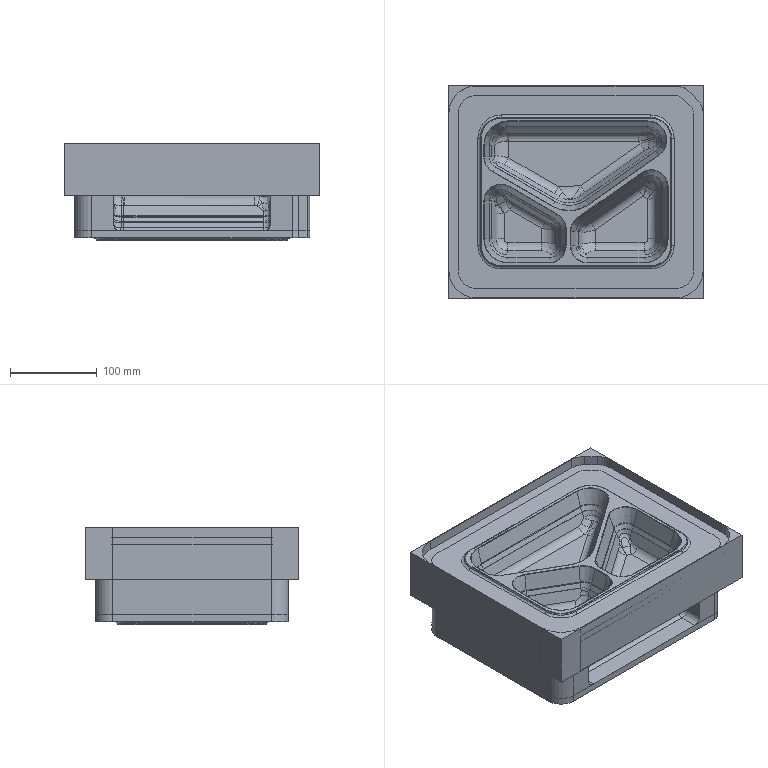NC program | NX | posted with a generic post | part box 295.651 x 246.652 x 112.895 mm
Lines 269047 to 269786 of 299251:
(D5 , TOOL : D10)
N538074 M6
N538076 G53
N538078 G17 G0 G90 X140.272 Y-100.089 S7000 M3 M8
N538080 G43 Z210.5 H0
N538082 Z50.884
N538084 G94 G1 X139.255 Y-102.613 Z50.741 F4000.
N538086 X137.526 Y-105.653 Z50.558
N538088 X135.406 Y-108.434 Z50.375
N538090 X132.933 Y-110.906 Z50.192
N538092 X130.152 Y-113.026 Z50.008
N538094 X127.113 Y-114.755 Z49.825
N538096 X123.869 Y-116.063 Z49.642
N538098 X120.48 Y-116.925 Z49.459
N538100 X117.007 Y-117.326 Z49.275
N538102 X109.541 Z48.884
N538104 X-115.756
N538106 G2 X-141.826 Y-91.256 R26.07
N538108 G1 Y91.256
N538110 G2 X-115.756 Y117.326 R26.07
N538112 G1 X115.613
N538114 G2 X126.951 Y112.629 R16.035
N538116 G1 X137.129 Y102.452
N538118 G2 X141.826 Y91.113 R16.035
N538120 G1 Y-91.256
N538122 G2 X115.756 Y-117.326 R26.07
N538124 G1 X109.541
N538126 Y-110.326
N538128 X-115.756
N538130 G2 X-134.826 Y-91.256 R19.07
N538132 G1 Y91.256
N538134 G2 X-115.756 Y110.326 R19.07
N538136 G1 X115.613
N538138 G2 X122.002 Y107.68 R9.035
N538140 G1 X132.179 Y97.502
N538142 G2 X134.826 Y91.113 R9.035
N538144 G1 Y-91.256
N538146 G2 X115.756 Y-110.326 R19.07
N538148 G1 X109.541
N538150 Y-103.326
N538152 X-115.756
N538154 G2 X-127.826 Y-91.256 R12.07
N538156 G1 Y91.256
N538158 G2 X-115.756 Y103.326 R12.07
N538160 G1 X115.613
N538162 G2 X117.052 Y102.73 R2.035
N538164 G1 X127.23 Y92.552
N538166 G2 X127.826 Y91.113 R2.035
N538168 G1 Y-91.256
N538170 G2 X115.756 Y-103.326 R12.07
N538172 G1 X109.541
N538174 Y-96.326
N538176 X-115.756
N538178 G2 X-120.826 Y-91.256 R5.07
N538180 G1 Y-80.756
N538182 X-113.826
N538184 G3 X-105.256 Y-89.326 R33.145
N538186 G1 X-113.826
N538188 Y-80.756
N538190 X-120.826
N538192 Y91.256
N538194 G2 X-115.756 Y96.326 R5.07
N538196 G1 X-105.256
N538198 Y89.326
N538200 G3 X-113.826 Y80.756 R33.145
N538202 G1 Y89.326
N538204 X-105.256
N538206 Y96.326
N538208 X113.556
N538210 X120.826 Y89.057
N538212 Y80.756
N538214 X113.826
N538216 G3 X105.256 Y89.326 R33.145
N538218 G1 X110.657
N538220 X113.826 Y86.157
N538222 Y80.756
N538224 X120.826
N538226 Y-91.256
N538228 G2 X115.756 Y-96.326 R5.07
N538230 G1 X109.541
N538232 Y-89.326
N538234 X105.256
N538236 G3 X113.826 Y-80.756 R33.145
N538238 G1 X112.671 Y-79.964
N538240 G2 X86.499 Y-93.744 R31.745
N538242 G1 X-86.499
N538244 G2 X-118.244 Y-61.999 R31.745
N538246 G1 Y61.999
N538248 G2 X-86.499 Y93.744 R31.745
N538250 G1 X86.499
N538252 G2 X118.244 Y61.999 R31.745
N538254 G1 Y-61.999
N538256 G2 X112.671 Y-79.964 R31.745
N538258 G1 X113.826 Y-80.756
N538260 Y-89.326
N538262 X109.541
N538264 G3 X107.541 Y-91.326 R2.
N538266 G1 Z49.884
N538268 G0 Z210.5
(D6 , TOOL : D10)
N538270 X-140.826 Y-74.472
N538272 Z49.884
N538274 G1 Y92.483 Z49.738
N538276 X-140.437 Y95.819 Z49.735
N538278 X-139.607 Y99.073 Z49.733
N538280 X-138.35 Y102.188 Z49.73
N538282 X-136.688 Y105.106 Z49.727
N538284 X-134.652 Y107.777 Z49.724
N538286 X-132.277 Y110.152 Z49.721
N538288 X-129.606 Y112.189 Z49.718
N538290 X-126.687 Y113.85 Z49.715
N538292 X-123.573 Y115.108 Z49.712
N538294 X-120.319 Y115.938 Z49.709
N538296 X-116.982 Y116.326 Z49.706
N538298 X116.563 Z49.502
N538300 X119.017 Y115.966 Z49.5
N538302 X121.378 Y115.209 Z49.498
N538304 X123.583 Y114.075 Z49.496
N538306 X125.572 Y112.594 Z49.494
N538308 X137.094 Y101.073 Z49.479
N538310 X138.575 Y99.084 Z49.477
N538312 X139.709 Y96.878 Z49.475
N538314 X140.466 Y94.517 Z49.473
N538316 X140.826 Y92.064 Z49.471
N538318 Y-92.483 Z49.31
N538320 X140.437 Y-95.819 Z49.307
N538322 X139.607 Y-99.073 Z49.304
N538324 X138.35 Y-102.188 Z49.301
N538326 X136.688 Y-105.106 Z49.298
N538328 X134.652 Y-107.777 Z49.295
N538330 X132.277 Y-110.152 Z49.292
N538332 X129.606 Y-112.189 Z49.289
N538334 X126.687 Y-113.85 Z49.286
N538336 X123.573 Y-115.108 Z49.283
N538338 X120.319 Y-115.938 Z49.28
N538340 X116.982 Y-116.326 Z49.278
N538342 X-116.982 Z49.073
N538344 X-120.319 Y-115.938 Z49.07
N538346 X-123.573 Y-115.108 Z49.067
N538348 X-126.687 Y-113.85 Z49.065
N538350 X-129.606 Y-112.189 Z49.062
N538352 X-132.277 Y-110.152 Z49.059
N538354 X-134.652 Y-107.777 Z49.056
N538356 X-136.688 Y-105.106 Z49.053
N538358 X-138.35 Y-102.188 Z49.05
N538360 X-139.607 Y-99.073 Z49.047
N538362 X-140.437 Y-95.819 Z49.044
N538364 X-140.826 Y-92.483 Z49.041
N538366 Y92.483 Z48.88
N538368 X-140.437 Y95.819 Z48.877
N538370 X-139.607 Y99.073 Z48.874
N538372 X-138.35 Y102.188 Z48.871
N538374 X-136.688 Y105.106 Z48.868
N538376 X-134.652 Y107.777 Z48.865
N538378 X-132.277 Y110.152 Z48.862
N538380 X-129.606 Y112.189 Z48.859
N538382 X-126.687 Y113.85 Z48.856
N538384 X-123.573 Y115.108 Z48.853
N538386 X-120.319 Y115.938 Z48.85
N538388 X-116.982 Y116.326 Z48.847
N538390 X116.563 Z48.644
N538392 X119.017 Y115.966 Z48.641
N538394 X121.378 Y115.209 Z48.639
N538396 X123.583 Y114.075 Z48.637
N538398 X125.572 Y112.594 Z48.635
N538400 X137.094 Y101.073 Z48.621
N538402 X138.575 Y99.084 Z48.619
N538404 X139.709 Y96.878 Z48.616
N538406 X140.466 Y94.517 Z48.614
N538408 X140.826 Y92.064 Z48.612
N538410 Y-92.483 Z48.451
N538412 X140.437 Y-95.819 Z48.448
N538414 X139.607 Y-99.073 Z48.445
N538416 X138.35 Y-102.188 Z48.442
N538418 X136.688 Y-105.106 Z48.439
N538420 X134.652 Y-107.777 Z48.436
N538422 X132.277 Y-110.152 Z48.433
N538424 X129.606 Y-112.189 Z48.431
N538426 X126.687 Y-113.85 Z48.428
N538428 X123.573 Y-115.108 Z48.425
N538430 X120.319 Y-115.938 Z48.422
N538432 X116.982 Y-116.326 Z48.419
N538434 X-116.982 Z48.215
N538436 X-120.319 Y-115.938 Z48.212
N538438 X-123.573 Y-115.108 Z48.209
N538440 X-126.687 Y-113.85 Z48.206
N538442 X-129.606 Y-112.189 Z48.203
N538444 X-132.277 Y-110.152 Z48.2
N538446 X-134.652 Y-107.777 Z48.197
N538448 X-136.688 Y-105.106 Z48.194
N538450 X-138.35 Y-102.188 Z48.191
N538452 X-139.607 Y-99.073 Z48.188
N538454 X-140.437 Y-95.819 Z48.185
N538456 X-140.826 Y-92.483 Z48.182
N538458 Y92.483 Z48.021
N538460 X-140.437 Y95.819 Z48.018
N538462 X-139.607 Y99.073 Z48.015
N538464 X-138.35 Y102.188 Z48.012
N538466 X-136.688 Y105.106 Z48.009
N538468 X-134.652 Y107.777 Z48.006
N538470 X-132.277 Y110.152 Z48.003
N538472 X-129.606 Y112.189 Z48.
N538474 X-126.687 Y113.85 Z47.998
N538476 X-123.573 Y115.108 Z47.995
N538478 X-120.319 Y115.938 Z47.992
N538480 X-116.982 Y116.326 Z47.989
N538482 X116.563 Z47.785
N538484 X119.017 Y115.966 Z47.783
N538486 X121.378 Y115.209 Z47.781
N538488 X123.583 Y114.075 Z47.778
N538490 X125.572 Y112.594 Z47.776
N538492 X137.094 Y101.073 Z47.762
N538494 X138.575 Y99.084 Z47.76
N538496 X139.709 Y96.878 Z47.758
N538498 X140.466 Y94.517 Z47.756
N538500 X140.826 Y92.064 Z47.753
N538502 Y-92.483 Z47.592
N538504 X140.437 Y-95.819 Z47.589
N538506 X139.607 Y-99.073 Z47.587
N538508 X138.35 Y-102.188 Z47.584
N538510 X136.688 Y-105.106 Z47.581
N538512 X134.652 Y-107.777 Z47.578
N538514 X132.277 Y-110.152 Z47.575
N538516 X129.606 Y-112.189 Z47.572
N538518 X126.687 Y-113.85 Z47.569
N538520 X123.573 Y-115.108 Z47.566
N538522 X120.319 Y-115.938 Z47.563
N538524 X116.982 Y-116.326 Z47.56
N538526 X-116.982 Z47.356
N538528 X-120.319 Y-115.938 Z47.353
N538530 X-123.573 Y-115.108 Z47.35
N538532 X-126.687 Y-113.85 Z47.347
N538534 X-129.606 Y-112.189 Z47.344
N538536 X-132.277 Y-110.152 Z47.341
N538538 X-134.652 Y-107.777 Z47.338
N538540 X-136.688 Y-105.106 Z47.335
N538542 X-138.35 Y-102.188 Z47.333
N538544 X-139.607 Y-99.073 Z47.33
N538546 X-140.437 Y-95.819 Z47.327
N538548 X-140.826 Y-92.483 Z47.324
N538550 Y92.483 Z47.162
N538552 X-140.437 Y95.819 Z47.159
N538554 X-139.607 Y99.073 Z47.156
N538556 X-138.35 Y102.188 Z47.154
N538558 X-136.688 Y105.106 Z47.151
N538560 X-134.652 Y107.777 Z47.148
N538562 X-132.277 Y110.152 Z47.145
N538564 X-129.606 Y112.189 Z47.142
N538566 X-126.687 Y113.85 Z47.139
N538568 X-123.573 Y115.108 Z47.136
N538570 X-120.319 Y115.938 Z47.133
N538572 X-116.982 Y116.326 Z47.13
N538574 X116.563 Z46.926
N538576 X119.017 Y115.966 Z46.924
N538578 X121.378 Y115.209 Z46.922
N538580 X123.583 Y114.075 Z46.92
N538582 X125.572 Y112.594 Z46.918
N538584 X137.094 Y101.073 Z46.903
N538586 X138.575 Y99.084 Z46.901
N538588 X139.709 Y96.878 Z46.899
N538590 X140.466 Y94.517 Z46.897
N538592 X140.826 Y92.064 Z46.895
N538594 Y-92.483 Z46.734
N538596 X140.437 Y-95.819 Z46.731
N538598 X139.607 Y-99.073 Z46.728
N538600 X138.35 Y-102.188 Z46.725
N538602 X136.688 Y-105.106 Z46.722
N538604 X134.652 Y-107.777 Z46.719
N538606 X132.277 Y-110.152 Z46.716
N538608 X129.606 Y-112.189 Z46.713
N538610 X126.687 Y-113.85 Z46.71
N538612 X123.573 Y-115.108 Z46.707
N538614 X120.319 Y-115.938 Z46.704
N538616 X116.982 Y-116.326 Z46.701
N538618 X-116.982 Z46.497
N538620 X-120.319 Y-115.938 Z46.494
N538622 X-123.573 Y-115.108 Z46.491
N538624 X-126.687 Y-113.85 Z46.488
N538626 X-129.606 Y-112.189 Z46.486
N538628 X-132.277 Y-110.152 Z46.483
N538630 X-134.652 Y-107.777 Z46.48
N538632 X-136.688 Y-105.106 Z46.477
N538634 X-138.35 Y-102.188 Z46.474
N538636 X-139.607 Y-99.073 Z46.471
N538638 X-140.437 Y-95.819 Z46.468
N538640 X-140.826 Y-92.483 Z46.465
N538642 Y92.483 Z46.304
N538644 X-140.437 Y95.819 Z46.301
N538646 X-139.607 Y99.073 Z46.298
N538648 X-138.35 Y102.188 Z46.295
N538650 X-136.688 Y105.106 Z46.292
N538652 X-134.652 Y107.777 Z46.289
N538654 X-132.277 Y110.152 Z46.286
N538656 X-129.606 Y112.189 Z46.283
N538658 X-126.687 Y113.85 Z46.28
N538660 X-123.573 Y115.108 Z46.277
N538662 X-120.319 Y115.938 Z46.274
N538664 X-116.982 Y116.326 Z46.271
N538666 X116.563 Z46.068
N538668 X119.017 Y115.966 Z46.065
N538670 X121.378 Y115.209 Z46.063
N538672 X123.583 Y114.075 Z46.061
N538674 X125.572 Y112.594 Z46.059
N538676 X137.094 Y101.073 Z46.045
N538678 X138.575 Y99.084 Z46.043
N538680 X139.709 Y96.878 Z46.04
N538682 X140.466 Y94.517 Z46.038
N538684 X140.826 Y92.064 Z46.036
N538686 Y-92.483 Z45.875
N538688 X140.437 Y-95.819 Z45.872
N538690 X139.607 Y-99.073 Z45.869
N538692 X138.35 Y-102.188 Z45.866
N538694 X136.688 Y-105.106 Z45.863
N538696 X134.652 Y-107.777 Z45.86
N538698 X132.277 Y-110.152 Z45.857
N538700 X129.606 Y-112.189 Z45.854
N538702 X126.687 Y-113.85 Z45.852
N538704 X123.573 Y-115.108 Z45.849
N538706 X120.319 Y-115.938 Z45.846
N538708 X116.982 Y-116.326 Z45.843
N538710 X-116.982 Z45.639
N538712 X-120.319 Y-115.938 Z45.636
N538714 X-123.573 Y-115.108 Z45.633
N538716 X-126.687 Y-113.85 Z45.63
N538718 X-129.606 Y-112.189 Z45.627
N538720 X-132.277 Y-110.152 Z45.624
N538722 X-134.652 Y-107.777 Z45.621
N538724 X-136.688 Y-105.106 Z45.618
N538726 X-138.35 Y-102.188 Z45.615
N538728 X-139.607 Y-99.073 Z45.612
N538730 X-140.437 Y-95.819 Z45.609
N538732 X-140.826 Y-92.483 Z45.606
N538734 Y92.483 Z45.445
N538736 X-140.437 Y95.819 Z45.442
N538738 X-139.607 Y99.073 Z45.439
N538740 X-138.35 Y102.188 Z45.436
N538742 X-136.688 Y105.106 Z45.433
N538744 X-134.652 Y107.777 Z45.43
N538746 X-132.277 Y110.152 Z45.427
N538748 X-129.606 Y112.189 Z45.424
N538750 X-126.687 Y113.85 Z45.421
N538752 X-123.573 Y115.108 Z45.419
N538754 X-120.319 Y115.938 Z45.416
N538756 X-116.982 Y116.326 Z45.413
N538758 X116.563 Z45.209
N538760 X119.017 Y115.966 Z45.207
N538762 X121.378 Y115.209 Z45.205
N538764 X123.583 Y114.075 Z45.202
N538766 X125.572 Y112.594 Z45.2
N538768 X137.094 Y101.073 Z45.186
N538770 X138.575 Y99.084 Z45.184
N538772 X139.709 Y96.878 Z45.182
N538774 X140.466 Y94.517 Z45.18
N538776 X140.826 Y92.064 Z45.177
N538778 Y-92.483 Z45.016
N538780 X140.437 Y-95.819 Z45.013
N538782 X139.607 Y-99.073 Z45.01
N538784 X138.35 Y-102.188 Z45.008
N538786 X136.688 Y-105.106 Z45.005
N538788 X134.652 Y-107.777 Z45.002
N538790 X132.277 Y-110.152 Z44.999
N538792 X129.606 Y-112.189 Z44.996
N538794 X126.687 Y-113.85 Z44.993
N538796 X123.573 Y-115.108 Z44.99
N538798 X120.319 Y-115.938 Z44.987
N538800 X116.982 Y-116.326 Z44.984
N538802 X-116.982 Z44.78
N538804 X-120.319 Y-115.938 Z44.777
N538806 X-123.573 Y-115.108 Z44.774
N538808 X-126.687 Y-113.85 Z44.771
N538810 X-129.606 Y-112.189 Z44.768
N538812 X-132.277 Y-110.152 Z44.765
N538814 X-134.652 Y-107.777 Z44.762
N538816 X-136.688 Y-105.106 Z44.759
N538818 X-138.35 Y-102.188 Z44.756
N538820 X-139.607 Y-99.073 Z44.754
N538822 X-140.437 Y-95.819 Z44.751
N538824 X-140.826 Y-92.483 Z44.748
N538826 Y92.483 Z44.586
N538828 X-140.437 Y95.819 Z44.583
N538830 X-139.607 Y99.073 Z44.58
N538832 X-138.35 Y102.188 Z44.577
N538834 X-136.688 Y105.106 Z44.575
N538836 X-134.652 Y107.777 Z44.572
N538838 X-132.277 Y110.152 Z44.569
N538840 X-129.606 Y112.189 Z44.566
N538842 X-126.687 Y113.85 Z44.563
N538844 X-123.573 Y115.108 Z44.56
N538846 X-120.319 Y115.938 Z44.557
N538848 X-116.982 Y116.326 Z44.554
N538850 X116.563 Z44.35
N538852 X119.017 Y115.966 Z44.348
N538854 X121.378 Y115.209 Z44.346
N538856 X123.583 Y114.075 Z44.344
N538858 X125.572 Y112.594 Z44.342
N538860 X137.094 Y101.073 Z44.327
N538862 X138.575 Y99.084 Z44.325
N538864 X139.709 Y96.878 Z44.323
N538866 X140.466 Y94.517 Z44.321
N538868 X140.826 Y92.064 Z44.319
N538870 Y-92.483 Z44.158
N538872 X140.437 Y-95.819 Z44.155
N538874 X139.607 Y-99.073 Z44.152
N538876 X138.35 Y-102.188 Z44.149
N538878 X136.688 Y-105.106 Z44.146
N538880 X134.652 Y-107.777 Z44.143
N538882 X132.277 Y-110.152 Z44.14
N538884 X129.606 Y-112.189 Z44.137
N538886 X126.687 Y-113.85 Z44.134
N538888 X123.573 Y-115.108 Z44.131
N538890 X120.319 Y-115.938 Z44.128
N538892 X116.982 Y-116.326 Z44.125
N538894 X-116.982 Z43.921
N538896 X-120.319 Y-115.938 Z43.918
N538898 X-123.573 Y-115.108 Z43.915
N538900 X-126.687 Y-113.85 Z43.912
N538902 X-129.606 Y-112.189 Z43.909
N538904 X-132.277 Y-110.152 Z43.907
N538906 X-134.652 Y-107.777 Z43.904
N538908 X-136.688 Y-105.106 Z43.901
N538910 X-138.35 Y-102.188 Z43.898
N538912 X-139.607 Y-99.073 Z43.895
N538914 X-140.437 Y-95.819 Z43.892
N538916 X-140.826 Y-92.483 Z43.889
N538918 Y92.483 Z43.728
N538920 X-140.437 Y95.819 Z43.725
N538922 X-139.607 Y99.073 Z43.722
N538924 X-138.35 Y102.188 Z43.719
N538926 X-136.688 Y105.106 Z43.716
N538928 X-134.652 Y107.777 Z43.713
N538930 X-132.277 Y110.152 Z43.71
N538932 X-129.606 Y112.189 Z43.707
N538934 X-126.687 Y113.85 Z43.704
N538936 X-123.573 Y115.108 Z43.701
N538938 X-120.319 Y115.938 Z43.698
N538940 X-116.982 Y116.326 Z43.695
N538942 X116.563 Z43.492
N538944 X119.017 Y115.966 Z43.489
N538946 X121.378 Y115.209 Z43.487
N538948 X123.583 Y114.075 Z43.485
N538950 X125.572 Y112.594 Z43.483
N538952 X137.094 Y101.073 Z43.469
N538954 X138.575 Y99.084 Z43.466
N538956 X139.709 Y96.878 Z43.464
N538958 X140.466 Y94.517 Z43.462
N538960 X140.826 Y92.064 Z43.46
N538962 Y-92.483 Z43.299
N538964 X140.437 Y-95.819 Z43.296
N538966 X139.607 Y-99.073 Z43.293
N538968 X138.35 Y-102.188 Z43.29
N538970 X136.688 Y-105.106 Z43.287
N538972 X134.652 Y-107.777 Z43.284
N538974 X132.277 Y-110.152 Z43.281
N538976 X129.606 Y-112.189 Z43.278
N538978 X126.687 Y-113.85 Z43.275
N538980 X123.573 Y-115.108 Z43.273
N538982 X120.319 Y-115.938 Z43.27
N538984 X116.982 Y-116.326 Z43.267
N538986 X-116.982 Z43.063
N538988 X-120.319 Y-115.938 Z43.06
N538990 X-123.573 Y-115.108 Z43.057
N538992 X-126.687 Y-113.85 Z43.054
N538994 X-129.606 Y-112.189 Z43.051
N538996 X-132.277 Y-110.152 Z43.048
N538998 X-134.652 Y-107.777 Z43.045
N539000 X-136.688 Y-105.106 Z43.042
N539002 X-138.35 Y-102.188 Z43.039
N539004 X-139.607 Y-99.073 Z43.036
N539006 X-140.437 Y-95.819 Z43.033
N539008 X-140.826 Y-92.483 Z43.03
N539010 Y92.483 Z42.869
N539012 X-140.437 Y95.819 Z42.866
N539014 X-139.607 Y99.073 Z42.863
N539016 X-138.35 Y102.188 Z42.86
N539018 X-136.688 Y105.106 Z42.857
N539020 X-134.652 Y107.777 Z42.854
N539022 X-132.277 Y110.152 Z42.851
N539024 X-129.606 Y112.189 Z42.848
N539026 X-126.687 Y113.85 Z42.845
N539028 X-123.573 Y115.108 Z42.842
N539030 X-120.319 Y115.938 Z42.84
N539032 X-116.982 Y116.326 Z42.837
N539034 X116.563 Z42.633
N539036 X119.017 Y115.966 Z42.631
N539038 X121.378 Y115.209 Z42.628
N539040 X123.583 Y114.075 Z42.626
N539042 X125.572 Y112.594 Z42.624
N539044 X137.094 Y101.073 Z42.61
N539046 X138.575 Y99.084 Z42.608
N539048 X139.709 Y96.878 Z42.606
N539050 X140.466 Y94.517 Z42.603
N539052 X140.826 Y92.064 Z42.601
N539054 Y-92.483 Z42.44
N539056 X140.437 Y-95.819 Z42.437
N539058 X139.607 Y-99.073 Z42.434
N539060 X138.35 Y-102.188 Z42.431
N539062 X136.688 Y-105.106 Z42.429
N539064 X134.652 Y-107.777 Z42.426
N539066 X132.277 Y-110.152 Z42.423
N539068 X129.606 Y-112.189 Z42.42
N539070 X126.687 Y-113.85 Z42.417
N539072 X123.573 Y-115.108 Z42.414
N539074 X120.319 Y-115.938 Z42.411
N539076 X116.982 Y-116.326 Z42.408
N539078 X-116.982 Z42.204
N539080 X-120.319 Y-115.938 Z42.201
N539082 X-123.573 Y-115.108 Z42.198
N539084 X-126.687 Y-113.85 Z42.195
N539086 X-129.606 Y-112.189 Z42.192
N539088 X-132.277 Y-110.152 Z42.189
N539090 X-134.652 Y-107.777 Z42.186
N539092 X-136.688 Y-105.106 Z42.183
N539094 X-138.35 Y-102.188 Z42.18
N539096 X-139.607 Y-99.073 Z42.177
N539098 X-140.437 Y-95.819 Z42.175
N539100 X-140.826 Y-92.483 Z42.172
N539102 Y92.483 Z42.01
N539104 X-140.437 Y95.819 Z42.007
N539106 X-139.607 Y99.073 Z42.004
N539108 X-138.35 Y102.188 Z42.001
N539110 X-136.688 Y105.106 Z41.998
N539112 X-134.652 Y107.777 Z41.996
N539114 X-132.277 Y110.152 Z41.993
N539116 X-129.606 Y112.189 Z41.99
N539118 X-126.687 Y113.85 Z41.987
N539120 X-123.573 Y115.108 Z41.984
N539122 X-120.319 Y115.938 Z41.981
N539124 X-116.982 Y116.326 Z41.978
N539126 X116.563 Z41.774
N539128 X119.017 Y115.966 Z41.772
N539130 X121.378 Y115.209 Z41.77
N539132 X123.583 Y114.075 Z41.768
N539134 X125.572 Y112.594 Z41.765
N539136 X137.094 Y101.073 Z41.751
N539138 X138.575 Y99.084 Z41.749
N539140 X139.709 Y96.878 Z41.747
N539142 X140.466 Y94.517 Z41.745
N539144 X140.826 Y92.064 Z41.743
N539146 Y-92.483 Z41.582
N539148 X140.437 Y-95.819 Z41.579
N539150 X139.607 Y-99.073 Z41.576
N539152 X138.35 Y-102.188 Z41.573
N539154 X136.688 Y-105.106 Z41.57
N539156 X134.652 Y-107.777 Z41.567
N539158 X132.277 Y-110.152 Z41.564
N539160 X129.606 Y-112.189 Z41.561
N539162 X126.687 Y-113.85 Z41.558
N539164 X123.573 Y-115.108 Z41.555
N539166 X120.319 Y-115.938 Z41.552
N539168 X116.982 Y-116.326 Z41.549
N539170 X-116.982 Z41.345
N539172 X-120.319 Y-115.938 Z41.342
N539174 X-123.573 Y-115.108 Z41.339
N539176 X-126.687 Y-113.85 Z41.336
N539178 X-129.606 Y-112.189 Z41.333
N539180 X-132.277 Y-110.152 Z41.33
N539182 X-134.652 Y-107.777 Z41.328
N539184 X-136.688 Y-105.106 Z41.325
N539186 X-138.35 Y-102.188 Z41.322
N539188 X-139.607 Y-99.073 Z41.319
N539190 X-140.437 Y-95.819 Z41.316
N539192 X-140.826 Y-92.483 Z41.313
N539194 Y92.483 Z41.151
N539196 X-140.437 Y95.819 Z41.149
N539198 X-139.607 Y99.073 Z41.146
N539200 X-138.35 Y102.188 Z41.143
N539202 X-136.688 Y105.106 Z41.14
N539204 X-134.652 Y107.777 Z41.137
N539206 X-132.277 Y110.152 Z41.134
N539208 X-129.606 Y112.189 Z41.131
N539210 X-126.687 Y113.85 Z41.128
N539212 X-123.573 Y115.108 Z41.125
N539214 X-120.319 Y115.938 Z41.122
N539216 X-116.982 Y116.326 Z41.119
N539218 X116.563 Z40.915
N539220 X119.017 Y115.966 Z40.913
N539222 X121.378 Y115.209 Z40.911
N539224 X123.583 Y114.075 Z40.909
N539226 X125.572 Y112.594 Z40.907
N539228 X137.094 Y101.073 Z40.893
N539230 X138.575 Y99.084 Z40.89
N539232 X139.709 Y96.878 Z40.888
N539234 X140.466 Y94.517 Z40.886
N539236 X140.826 Y92.064 Z40.884
N539238 Y-92.483 Z40.723
N539240 X140.437 Y-95.819 Z40.72
N539242 X139.607 Y-99.073 Z40.717
N539244 X138.35 Y-102.188 Z40.714
N539246 X136.688 Y-105.106 Z40.711
N539248 X134.652 Y-107.777 Z40.708
N539250 X132.277 Y-110.152 Z40.705
N539252 X129.606 Y-112.189 Z40.702
N539254 X126.687 Y-113.85 Z40.699
N539256 X123.573 Y-115.108 Z40.696
N539258 X120.319 Y-115.938 Z40.694
N539260 X116.982 Y-116.326 Z40.691
N539262 X-116.982 Z40.486
N539264 X-120.319 Y-115.938 Z40.484
N539266 X-123.573 Y-115.108 Z40.481
N539268 X-126.687 Y-113.85 Z40.478
N539270 X-129.606 Y-112.189 Z40.475
N539272 X-132.277 Y-110.152 Z40.472
N539274 X-134.652 Y-107.777 Z40.469
N539276 X-136.688 Y-105.106 Z40.466
N539278 X-138.35 Y-102.188 Z40.463
N539280 X-139.607 Y-99.073 Z40.46
N539282 X-140.437 Y-95.819 Z40.457
N539284 X-140.826 Y-92.483 Z40.454
N539286 Y92.483 Z40.293
N539288 X-140.437 Y95.819 Z40.29
N539290 X-139.607 Y99.073 Z40.287
N539292 X-138.35 Y102.188 Z40.284
N539294 X-136.688 Y105.106 Z40.281
N539296 X-134.652 Y107.777 Z40.278
N539298 X-132.277 Y110.152 Z40.275
N539300 X-129.606 Y112.189 Z40.272
N539302 X-126.687 Y113.85 Z40.269
N539304 X-123.573 Y115.108 Z40.266
N539306 X-120.319 Y115.938 Z40.263
N539308 X-116.982 Y116.326 Z40.261
N539310 X116.563 Z40.057
N539312 X119.017 Y115.966 Z40.055
N539314 X121.378 Y115.209 Z40.052
N539316 X123.583 Y114.075 Z40.05
N539318 X125.572 Y112.594 Z40.048
N539320 X137.094 Y101.073 Z40.034
N539322 X138.575 Y99.084 Z40.032
N539324 X139.709 Y96.878 Z40.03
N539326 X140.466 Y94.517 Z40.027
N539328 X140.826 Y92.064 Z40.025
N539330 Y-92.483 Z39.864
N539332 X140.437 Y-95.819 Z39.861
N539334 X139.607 Y-99.073 Z39.858
N539336 X138.35 Y-102.188 Z39.855
N539338 X136.688 Y-105.106 Z39.852
N539340 X134.652 Y-107.777 Z39.85
N539342 X132.277 Y-110.152 Z39.847
N539344 X129.606 Y-112.189 Z39.844
N539346 X126.687 Y-113.85 Z39.841
N539348 X123.573 Y-115.108 Z39.838
N539350 X120.319 Y-115.938 Z39.835
N539352 X116.982 Y-116.326 Z39.832
N539354 X-116.982 Z39.628
N539356 X-120.319 Y-115.938 Z39.625
N539358 X-123.573 Y-115.108 Z39.622
N539360 X-126.687 Y-113.85 Z39.619
N539362 X-129.606 Y-112.189 Z39.616
N539364 X-132.277 Y-110.152 Z39.613
N539366 X-134.652 Y-107.777 Z39.61
N539368 X-136.688 Y-105.106 Z39.607
N539370 X-138.35 Y-102.188 Z39.604
N539372 X-139.607 Y-99.073 Z39.601
N539374 X-140.437 Y-95.819 Z39.598
N539376 X-140.826 Y-92.483 Z39.596
N539378 Y92.483 Z39.434
N539380 X-140.437 Y95.819 Z39.431
N539382 X-139.607 Y99.073 Z39.428
N539384 X-138.35 Y102.188 Z39.425
N539386 X-136.688 Y105.106 Z39.422
N539388 X-134.652 Y107.777 Z39.419
N539390 X-132.277 Y110.152 Z39.417
N539392 X-129.606 Y112.189 Z39.414
N539394 X-126.687 Y113.85 Z39.411
N539396 X-123.573 Y115.108 Z39.408
N539398 X-120.319 Y115.938 Z39.405
N539400 X-116.982 Y116.326 Z39.402
N539402 X116.563 Z39.198
N539404 X119.017 Y115.966 Z39.196
N539406 X121.378 Y115.209 Z39.194
N539408 X123.583 Y114.075 Z39.192
N539410 X125.572 Y112.594 Z39.189
N539412 X137.094 Y101.073 Z39.175
N539414 X138.575 Y99.084 Z39.173
N539416 X139.709 Y96.878 Z39.171
N539418 X140.466 Y94.517 Z39.169
N539420 X140.826 Y92.064 Z39.167
N539422 Y-92.483 Z39.005
N539424 X140.437 Y-95.819 Z39.003
N539426 X139.607 Y-99.073 Z39.
N539428 X138.35 Y-102.188 Z38.997
N539430 X136.688 Y-105.106 Z38.994
N539432 X134.652 Y-107.777 Z38.991
N539434 X132.277 Y-110.152 Z38.988
N539436 X129.606 Y-112.189 Z38.985
N539438 X126.687 Y-113.85 Z38.982
N539440 X123.573 Y-115.108 Z38.979
N539442 X120.319 Y-115.938 Z38.976
N539444 X116.982 Y-116.326 Z38.973
N539446 X-116.982 Z38.769
N539448 X-120.319 Y-115.938 Z38.766
N539450 X-123.573 Y-115.108 Z38.763
N539452 X-126.687 Y-113.85 Z38.76
N539454 X-129.606 Y-112.189 Z38.757
N539456 X-132.277 Y-110.152 Z38.754
N539458 X-134.652 Y-107.777 Z38.751
N539460 X-136.688 Y-105.106 Z38.749
N539462 X-138.35 Y-102.188 Z38.746
N539464 X-139.607 Y-99.073 Z38.743
N539466 X-140.437 Y-95.819 Z38.74
N539468 X-140.826 Y-92.483 Z38.737
N539470 Y92.483 Z38.575
N539472 X-140.437 Y95.819 Z38.572
N539474 X-139.607 Y99.073 Z38.57
N539476 X-138.35 Y102.188 Z38.567
N539478 X-136.688 Y105.106 Z38.564
N539480 X-134.652 Y107.777 Z38.561
N539482 X-132.277 Y110.152 Z38.558
N539484 X-129.606 Y112.189 Z38.555
N539486 X-126.687 Y113.85 Z38.552
N539488 X-123.573 Y115.108 Z38.549
N539490 X-120.319 Y115.938 Z38.546
N539492 X-116.982 Y116.326 Z38.543
N539494 X116.563 Z38.339
N539496 X119.017 Y115.966 Z38.337
N539498 X121.378 Y115.209 Z38.335
N539500 X123.583 Y114.075 Z38.333
N539502 X125.572 Y112.594 Z38.331
N539504 X137.094 Y101.073 Z38.316
N539506 X138.575 Y99.084 Z38.314
N539508 X139.709 Y96.878 Z38.312
N539510 X140.466 Y94.517 Z38.31
N539512 X140.826 Y92.064 Z38.308
N539514 Y-92.483 Z38.147
N539516 X140.437 Y-95.819 Z38.144
N539518 X139.607 Y-99.073 Z38.141
N539520 X138.35 Y-102.188 Z38.138
N539522 X136.688 Y-105.106 Z38.135
N539524 X134.652 Y-107.777 Z38.132
N539526 X132.277 Y-110.152 Z38.129
N539528 X129.606 Y-112.189 Z38.126
N539530 X126.687 Y-113.85 Z38.123
N539532 X123.573 Y-115.108 Z38.12
N539534 X120.319 Y-115.938 Z38.117
N539536 X116.982 Y-116.326 Z38.115
N539538 X-116.982 Z37.91
N539540 X-120.319 Y-115.938 Z37.907